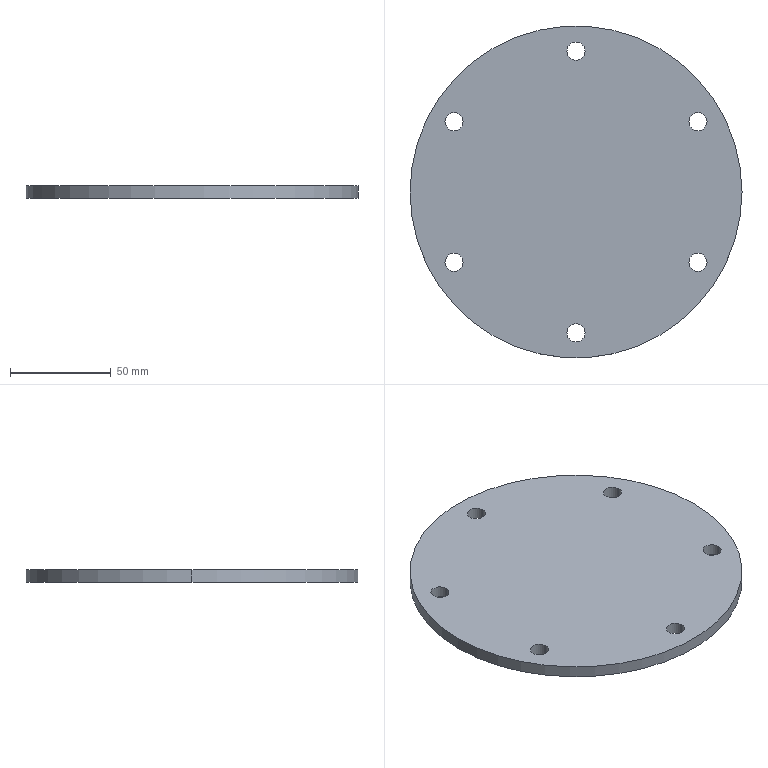Part | SolidWorks | features FlatPattern 1, SMBaseFlange 1, SheetMetal 1 | 1 solid | 16 faces | box 165 x 165 x 6 mm | volume 126005 mm3 | cylinder 14 | plane 2 | commonest cylinder face diameters 9 x12 165 x2
STEP:
#1=CARTESIAN_POINT('',(-65.122,35.,6.));
#2=VERTEX_POINT('',#1);
#3=CARTESIAN_POINT('',(-56.122,35.,6.));
#4=VERTEX_POINT('',#3);
#5=CARTESIAN_POINT('',(-60.622,35.,6.));
#6=DIRECTION('',(0.,0.,1.));
#7=DIRECTION('',(1.,0.,0.));
#8=AXIS2_PLACEMENT_3D('',#5,#6,#7);
#9=CIRCLE('',#8,4.5);
#10=EDGE_CURVE('',#2,#4,#9,.T.);
#11=ORIENTED_EDGE('',*,*,#10,.T.);
#12=CARTESIAN_POINT('',(-56.122,35.,0.));
#13=VERTEX_POINT('',#12);
#14=CARTESIAN_POINT('',(-56.122,35.,6.));
#15=DIRECTION('',(0.,0.,-1.));
#16=VECTOR('',#15,1000.);
#17=LINE('',#14,#16);
#18=EDGE_CURVE('',#4,#13,#17,.T.);
#19=ORIENTED_EDGE('',*,*,#18,.T.);
#20=CARTESIAN_POINT('',(-65.122,35.,0.));
#21=VERTEX_POINT('',#20);
#22=CARTESIAN_POINT('',(-60.622,35.,0.));
#23=DIRECTION('',(0.,0.,1.));
#24=DIRECTION('',(1.,0.,0.));
#25=AXIS2_PLACEMENT_3D('',#22,#23,#24);
#26=CIRCLE('',#25,4.5);
#27=EDGE_CURVE('',#21,#13,#26,.T.);
#28=ORIENTED_EDGE('',*,*,#27,.F.);
#29=CARTESIAN_POINT('',(-65.122,35.,6.));
#30=DIRECTION('',(0.,0.,-1.));
#31=VECTOR('',#30,1000.);
#32=LINE('',#29,#31);
#33=EDGE_CURVE('',#2,#21,#32,.T.);
#34=ORIENTED_EDGE('',*,*,#33,.F.);
#35=EDGE_LOOP('',(#11,#19,#28,#34));
#36=FACE_OUTER_BOUND('',#35,.T.);
#37=CARTESIAN_POINT('',(-60.622,35.,6.));
#38=DIRECTION('',(0.,0.,-1.));
#39=DIRECTION('',(-1.,0.,0.));
#40=AXIS2_PLACEMENT_3D('',#37,#38,#39);
#41=CYLINDRICAL_SURFACE('',#40,4.5);
#42=ADVANCED_FACE('',(#36),#41,.F.);
#43=CARTESIAN_POINT('',(-65.122,-35.,6.));
#44=VERTEX_POINT('',#43);
#45=CARTESIAN_POINT('',(-56.122,-35.,6.));
#46=VERTEX_POINT('',#45);
#47=CARTESIAN_POINT('',(-60.622,-35.,6.));
#48=DIRECTION('',(0.,0.,1.));
#49=DIRECTION('',(1.,0.,0.));
#50=AXIS2_PLACEMENT_3D('',#47,#48,#49);
#51=CIRCLE('',#50,4.5);
#52=EDGE_CURVE('',#44,#46,#51,.T.);
#53=ORIENTED_EDGE('',*,*,#52,.T.);
#54=CARTESIAN_POINT('',(-56.122,-35.,0.));
#55=VERTEX_POINT('',#54);
#56=CARTESIAN_POINT('',(-56.122,-35.,6.));
#57=DIRECTION('',(0.,0.,-1.));
#58=VECTOR('',#57,1000.);
#59=LINE('',#56,#58);
#60=EDGE_CURVE('',#46,#55,#59,.T.);
#61=ORIENTED_EDGE('',*,*,#60,.T.);
#62=CARTESIAN_POINT('',(-65.122,-35.,0.));
#63=VERTEX_POINT('',#62);
#64=CARTESIAN_POINT('',(-60.622,-35.,0.));
#65=DIRECTION('',(0.,0.,1.));
#66=DIRECTION('',(1.,0.,0.));
#67=AXIS2_PLACEMENT_3D('',#64,#65,#66);
#68=CIRCLE('',#67,4.5);
#69=EDGE_CURVE('',#63,#55,#68,.T.);
#70=ORIENTED_EDGE('',*,*,#69,.F.);
#71=CARTESIAN_POINT('',(-65.122,-35.,6.));
#72=DIRECTION('',(0.,0.,-1.));
#73=VECTOR('',#72,1000.);
#74=LINE('',#71,#73);
#75=EDGE_CURVE('',#44,#63,#74,.T.);
#76=ORIENTED_EDGE('',*,*,#75,.F.);
#77=EDGE_LOOP('',(#53,#61,#70,#76));
#78=FACE_OUTER_BOUND('',#77,.T.);
#79=CARTESIAN_POINT('',(-60.622,-35.,6.));
#80=DIRECTION('',(0.,0.,-1.));
#81=DIRECTION('',(-1.,0.,0.));
#82=AXIS2_PLACEMENT_3D('',#79,#80,#81);
#83=CYLINDRICAL_SURFACE('',#82,4.5);
#84=ADVANCED_FACE('',(#78),#83,.F.);
#85=CARTESIAN_POINT('',(-4.5,-70.,6.));
#86=VERTEX_POINT('',#85);
#87=CARTESIAN_POINT('',(4.5,-70.,6.));
#88=VERTEX_POINT('',#87);
#89=CARTESIAN_POINT('',(0.,-70.,6.));
#90=DIRECTION('',(0.,0.,1.));
#91=DIRECTION('',(1.,0.,0.));
#92=AXIS2_PLACEMENT_3D('',#89,#90,#91);
#93=CIRCLE('',#92,4.5);
#94=EDGE_CURVE('',#86,#88,#93,.T.);
#95=ORIENTED_EDGE('',*,*,#94,.T.);
#96=CARTESIAN_POINT('',(4.5,-70.,0.));
#97=VERTEX_POINT('',#96);
#98=CARTESIAN_POINT('',(4.5,-70.,6.));
#99=DIRECTION('',(0.,0.,-1.));
#100=VECTOR('',#99,1000.);
#101=LINE('',#98,#100);
#102=EDGE_CURVE('',#88,#97,#101,.T.);
#103=ORIENTED_EDGE('',*,*,#102,.T.);
#104=CARTESIAN_POINT('',(-4.5,-70.,0.));
#105=VERTEX_POINT('',#104);
#106=CARTESIAN_POINT('',(0.,-70.,0.));
#107=DIRECTION('',(0.,0.,1.));
#108=DIRECTION('',(1.,0.,0.));
#109=AXIS2_PLACEMENT_3D('',#106,#107,#108);
#110=CIRCLE('',#109,4.5);
#111=EDGE_CURVE('',#105,#97,#110,.T.);
#112=ORIENTED_EDGE('',*,*,#111,.F.);
#113=CARTESIAN_POINT('',(-4.5,-70.,6.));
#114=DIRECTION('',(0.,0.,-1.));
#115=VECTOR('',#114,1000.);
#116=LINE('',#113,#115);
#117=EDGE_CURVE('',#86,#105,#116,.T.);
#118=ORIENTED_EDGE('',*,*,#117,.F.);
#119=EDGE_LOOP('',(#95,#103,#112,#118));
#120=FACE_OUTER_BOUND('',#119,.T.);
#121=CARTESIAN_POINT('',(0.,-70.,6.));
#122=DIRECTION('',(0.,0.,-1.));
#123=DIRECTION('',(-1.,0.,0.));
#124=AXIS2_PLACEMENT_3D('',#121,#122,#123);
#125=CYLINDRICAL_SURFACE('',#124,4.5);
#126=ADVANCED_FACE('',(#120),#125,.F.);
#127=CARTESIAN_POINT('',(56.122,-35.,6.));
#128=VERTEX_POINT('',#127);
#129=CARTESIAN_POINT('',(65.122,-35.,6.));
#130=VERTEX_POINT('',#129);
#131=CARTESIAN_POINT('',(60.622,-35.,6.));
#132=DIRECTION('',(0.,0.,1.));
#133=DIRECTION('',(1.,0.,0.));
#134=AXIS2_PLACEMENT_3D('',#131,#132,#133);
#135=CIRCLE('',#134,4.5);
#136=EDGE_CURVE('',#128,#130,#135,.T.);
#137=ORIENTED_EDGE('',*,*,#136,.T.);
#138=CARTESIAN_POINT('',(65.122,-35.,0.));
#139=VERTEX_POINT('',#138);
#140=CARTESIAN_POINT('',(65.122,-35.,6.));
#141=DIRECTION('',(0.,0.,-1.));
#142=VECTOR('',#141,1000.);
#143=LINE('',#140,#142);
#144=EDGE_CURVE('',#130,#139,#143,.T.);
#145=ORIENTED_EDGE('',*,*,#144,.T.);
#146=CARTESIAN_POINT('',(56.122,-35.,0.));
#147=VERTEX_POINT('',#146);
#148=CARTESIAN_POINT('',(60.622,-35.,0.));
#149=DIRECTION('',(0.,0.,1.));
#150=DIRECTION('',(1.,0.,0.));
#151=AXIS2_PLACEMENT_3D('',#148,#149,#150);
#152=CIRCLE('',#151,4.5);
#153=EDGE_CURVE('',#147,#139,#152,.T.);
#154=ORIENTED_EDGE('',*,*,#153,.F.);
#155=CARTESIAN_POINT('',(56.122,-35.,6.));
#156=DIRECTION('',(0.,0.,-1.));
#157=VECTOR('',#156,1000.);
#158=LINE('',#155,#157);
#159=EDGE_CURVE('',#128,#147,#158,.T.);
#160=ORIENTED_EDGE('',*,*,#159,.F.);
#161=EDGE_LOOP('',(#137,#145,#154,#160));
#162=FACE_OUTER_BOUND('',#161,.T.);
#163=CARTESIAN_POINT('',(60.622,-35.,6.));
#164=DIRECTION('',(0.,0.,-1.));
#165=DIRECTION('',(-1.,0.,0.));
#166=AXIS2_PLACEMENT_3D('',#163,#164,#165);
#167=CYLINDRICAL_SURFACE('',#166,4.5);
#168=ADVANCED_FACE('',(#162),#167,.F.);
#169=CARTESIAN_POINT('',(56.122,35.,6.));
#170=VERTEX_POINT('',#169);
#171=CARTESIAN_POINT('',(65.122,35.,6.));
#172=VERTEX_POINT('',#171);
#173=CARTESIAN_POINT('',(60.622,35.,6.));
#174=DIRECTION('',(0.,0.,1.));
#175=DIRECTION('',(1.,0.,0.));
#176=AXIS2_PLACEMENT_3D('',#173,#174,#175);
#177=CIRCLE('',#176,4.5);
#178=EDGE_CURVE('',#170,#172,#177,.T.);
#179=ORIENTED_EDGE('',*,*,#178,.T.);
#180=CARTESIAN_POINT('',(65.122,35.,0.));
#181=VERTEX_POINT('',#180);
#182=CARTESIAN_POINT('',(65.122,35.,6.));
#183=DIRECTION('',(0.,0.,-1.));
#184=VECTOR('',#183,1000.);
#185=LINE('',#182,#184);
#186=EDGE_CURVE('',#172,#181,#185,.T.);
#187=ORIENTED_EDGE('',*,*,#186,.T.);
#188=CARTESIAN_POINT('',(56.122,35.,0.));
#189=VERTEX_POINT('',#188);
#190=CARTESIAN_POINT('',(60.622,35.,0.));
#191=DIRECTION('',(0.,0.,1.));
#192=DIRECTION('',(1.,0.,0.));
#193=AXIS2_PLACEMENT_3D('',#190,#191,#192);
#194=CIRCLE('',#193,4.5);
#195=EDGE_CURVE('',#189,#181,#194,.T.);
#196=ORIENTED_EDGE('',*,*,#195,.F.);
#197=CARTESIAN_POINT('',(56.122,35.,6.));
#198=DIRECTION('',(0.,0.,-1.));
#199=VECTOR('',#198,1000.);
#200=LINE('',#197,#199);
#201=EDGE_CURVE('',#170,#189,#200,.T.);
#202=ORIENTED_EDGE('',*,*,#201,.F.);
#203=EDGE_LOOP('',(#179,#187,#196,#202));
#204=FACE_OUTER_BOUND('',#203,.T.);
#205=CARTESIAN_POINT('',(60.622,35.,6.));
#206=DIRECTION('',(0.,0.,-1.));
#207=DIRECTION('',(-1.,0.,0.));
#208=AXIS2_PLACEMENT_3D('',#205,#206,#207);
#209=CYLINDRICAL_SURFACE('',#208,4.5);
#210=ADVANCED_FACE('',(#204),#209,.F.);
#211=CARTESIAN_POINT('',(-4.5,70.,6.));
#212=VERTEX_POINT('',#211);
#213=CARTESIAN_POINT('',(4.5,70.,6.));
#214=VERTEX_POINT('',#213);
#215=CARTESIAN_POINT('',(0.,70.,6.));
#216=DIRECTION('',(0.,0.,1.));
#217=DIRECTION('',(1.,0.,0.));
#218=AXIS2_PLACEMENT_3D('',#215,#216,#217);
#219=CIRCLE('',#218,4.5);
#220=EDGE_CURVE('',#212,#214,#219,.T.);
#221=ORIENTED_EDGE('',*,*,#220,.T.);
#222=CARTESIAN_POINT('',(4.5,70.,0.));
#223=VERTEX_POINT('',#222);
#224=CARTESIAN_POINT('',(4.5,70.,6.));
#225=DIRECTION('',(0.,0.,-1.));
#226=VECTOR('',#225,1000.);
#227=LINE('',#224,#226);
#228=EDGE_CURVE('',#214,#223,#227,.T.);
#229=ORIENTED_EDGE('',*,*,#228,.T.);
#230=CARTESIAN_POINT('',(-4.5,70.,0.));
#231=VERTEX_POINT('',#230);
#232=CARTESIAN_POINT('',(0.,70.,0.));
#233=DIRECTION('',(0.,0.,1.));
#234=DIRECTION('',(1.,0.,0.));
#235=AXIS2_PLACEMENT_3D('',#232,#233,#234);
#236=CIRCLE('',#235,4.5);
#237=EDGE_CURVE('',#231,#223,#236,.T.);
#238=ORIENTED_EDGE('',*,*,#237,.F.);
#239=CARTESIAN_POINT('',(-4.5,70.,6.));
#240=DIRECTION('',(0.,0.,-1.));
#241=VECTOR('',#240,1000.);
#242=LINE('',#239,#241);
#243=EDGE_CURVE('',#212,#231,#242,.T.);
#244=ORIENTED_EDGE('',*,*,#243,.F.);
#245=EDGE_LOOP('',(#221,#229,#238,#244));
#246=FACE_OUTER_BOUND('',#245,.T.);
#247=CARTESIAN_POINT('',(0.,70.,6.));
#248=DIRECTION('',(0.,0.,-1.));
#249=DIRECTION('',(-1.,0.,0.));
#250=AXIS2_PLACEMENT_3D('',#247,#248,#249);
#251=CYLINDRICAL_SURFACE('',#250,4.5);
#252=ADVANCED_FACE('',(#246),#251,.F.);
#253=CARTESIAN_POINT('',(82.5,0.,6.));
#254=VERTEX_POINT('',#253);
#255=CARTESIAN_POINT('',(-82.5,0.,6.));
#256=VERTEX_POINT('',#255);
#257=CARTESIAN_POINT('',(0.,0.,6.));
#258=DIRECTION('',(0.,0.,1.));
#259=DIRECTION('',(1.,0.,0.));
#260=AXIS2_PLACEMENT_3D('',#257,#258,#259);
#261=CIRCLE('',#260,82.5);
#262=EDGE_CURVE('',#254,#256,#261,.T.);
#263=ORIENTED_EDGE('',*,*,#262,.F.);
#264=CARTESIAN_POINT('',(82.5,0.,0.));
#265=VERTEX_POINT('',#264);
#266=CARTESIAN_POINT('',(82.5,0.,6.));
#267=DIRECTION('',(0.,0.,-1.));
#268=VECTOR('',#267,1000.);
#269=LINE('',#266,#268);
#270=EDGE_CURVE('',#254,#265,#269,.T.);
#271=ORIENTED_EDGE('',*,*,#270,.T.);
#272=CARTESIAN_POINT('',(-82.5,0.,0.));
#273=VERTEX_POINT('',#272);
#274=CARTESIAN_POINT('',(0.,0.,0.));
#275=DIRECTION('',(0.,0.,1.));
#276=DIRECTION('',(1.,0.,0.));
#277=AXIS2_PLACEMENT_3D('',#274,#275,#276);
#278=CIRCLE('',#277,82.5);
#279=EDGE_CURVE('',#265,#273,#278,.T.);
#280=ORIENTED_EDGE('',*,*,#279,.T.);
#281=CARTESIAN_POINT('',(-82.5,0.,6.));
#282=DIRECTION('',(0.,0.,-1.));
#283=VECTOR('',#282,1000.);
#284=LINE('',#281,#283);
#285=EDGE_CURVE('',#256,#273,#284,.T.);
#286=ORIENTED_EDGE('',*,*,#285,.F.);
#287=EDGE_LOOP('',(#263,#271,#280,#286));
#288=FACE_OUTER_BOUND('',#287,.T.);
#289=CARTESIAN_POINT('',(0.,0.,6.));
#290=DIRECTION('',(0.,0.,-1.));
#291=DIRECTION('',(-1.,0.,0.));
#292=AXIS2_PLACEMENT_3D('',#289,#290,#291);
#293=CYLINDRICAL_SURFACE('',#292,82.5);
#294=ADVANCED_FACE('',(#288),#293,.T.);
#295=ORIENTED_EDGE('',*,*,#52,.F.);
#296=CARTESIAN_POINT('',(-60.622,-35.,6.));
#297=DIRECTION('',(0.,0.,1.));
#298=DIRECTION('',(1.,0.,0.));
#299=AXIS2_PLACEMENT_3D('',#296,#297,#298);
#300=CIRCLE('',#299,4.5);
#301=EDGE_CURVE('',#46,#44,#300,.T.);
#302=ORIENTED_EDGE('',*,*,#301,.F.);
#303=EDGE_LOOP('',(#295,#302));
#304=FACE_BOUND('',#303,.T.);
#305=ORIENTED_EDGE('',*,*,#136,.F.);
#306=CARTESIAN_POINT('',(60.622,-35.,6.));
#307=DIRECTION('',(0.,0.,1.));
#308=DIRECTION('',(1.,0.,0.));
#309=AXIS2_PLACEMENT_3D('',#306,#307,#308);
#310=CIRCLE('',#309,4.5);
#311=EDGE_CURVE('',#130,#128,#310,.T.);
#312=ORIENTED_EDGE('',*,*,#311,.F.);
#313=EDGE_LOOP('',(#305,#312));
#314=FACE_BOUND('',#313,.T.);
#315=ORIENTED_EDGE('',*,*,#220,.F.);
#316=CARTESIAN_POINT('',(0.,70.,6.));
#317=DIRECTION('',(0.,0.,1.));
#318=DIRECTION('',(1.,0.,0.));
#319=AXIS2_PLACEMENT_3D('',#316,#317,#318);
#320=CIRCLE('',#319,4.5);
#321=EDGE_CURVE('',#214,#212,#320,.T.);
#322=ORIENTED_EDGE('',*,*,#321,.F.);
#323=EDGE_LOOP('',(#315,#322));
#324=FACE_BOUND('',#323,.T.);
#325=CARTESIAN_POINT('',(0.,0.,6.));
#326=DIRECTION('',(0.,0.,1.));
#327=DIRECTION('',(1.,0.,0.));
#328=AXIS2_PLACEMENT_3D('',#325,#326,#327);
#329=CIRCLE('',#328,82.5);
#330=EDGE_CURVE('',#256,#254,#329,.T.);
#331=ORIENTED_EDGE('',*,*,#330,.T.);
#332=ORIENTED_EDGE('',*,*,#262,.T.);
#333=EDGE_LOOP('',(#331,#332));
#334=FACE_OUTER_BOUND('',#333,.T.);
#335=ORIENTED_EDGE('',*,*,#178,.F.);
#336=CARTESIAN_POINT('',(60.622,35.,6.));
#337=DIRECTION('',(0.,0.,1.));
#338=DIRECTION('',(1.,0.,0.));
#339=AXIS2_PLACEMENT_3D('',#336,#337,#338);
#340=CIRCLE('',#339,4.5);
#341=EDGE_CURVE('',#172,#170,#340,.T.);
#342=ORIENTED_EDGE('',*,*,#341,.F.);
#343=EDGE_LOOP('',(#335,#342));
#344=FACE_BOUND('',#343,.T.);
#345=ORIENTED_EDGE('',*,*,#94,.F.);
#346=CARTESIAN_POINT('',(0.,-70.,6.));
#347=DIRECTION('',(0.,0.,1.));
#348=DIRECTION('',(1.,0.,0.));
#349=AXIS2_PLACEMENT_3D('',#346,#347,#348);
#350=CIRCLE('',#349,4.5);
#351=EDGE_CURVE('',#88,#86,#350,.T.);
#352=ORIENTED_EDGE('',*,*,#351,.F.);
#353=EDGE_LOOP('',(#345,#352));
#354=FACE_BOUND('',#353,.T.);
#355=ORIENTED_EDGE('',*,*,#10,.F.);
#356=CARTESIAN_POINT('',(-60.622,35.,6.));
#357=DIRECTION('',(0.,0.,1.));
#358=DIRECTION('',(1.,0.,0.));
#359=AXIS2_PLACEMENT_3D('',#356,#357,#358);
#360=CIRCLE('',#359,4.5);
#361=EDGE_CURVE('',#4,#2,#360,.T.);
#362=ORIENTED_EDGE('',*,*,#361,.F.);
#363=EDGE_LOOP('',(#355,#362));
#364=FACE_BOUND('',#363,.T.);
#365=CARTESIAN_POINT('',(0.,0.,6.));
#366=DIRECTION('',(0.,0.,1.));
#367=DIRECTION('',(1.,0.,0.));
#368=AXIS2_PLACEMENT_3D('',#365,#366,#367);
#369=PLANE('',#368);
#370=ADVANCED_FACE('',(#304,#314,#324,#334,#344,#354,#364),#369,.T.);
#371=CARTESIAN_POINT('',(0.,0.,0.));
#372=DIRECTION('',(0.,0.,1.));
#373=DIRECTION('',(1.,0.,0.));
#374=AXIS2_PLACEMENT_3D('',#371,#372,#373);
#375=CIRCLE('',#374,82.5);
#376=EDGE_CURVE('',#273,#265,#375,.T.);
#377=ORIENTED_EDGE('',*,*,#376,.F.);
#378=ORIENTED_EDGE('',*,*,#279,.F.);
#379=EDGE_LOOP('',(#377,#378));
#380=FACE_OUTER_BOUND('',#379,.T.);
#381=ORIENTED_EDGE('',*,*,#237,.T.);
#382=CARTESIAN_POINT('',(0.,70.,0.));
#383=DIRECTION('',(0.,0.,1.));
#384=DIRECTION('',(1.,0.,0.));
#385=AXIS2_PLACEMENT_3D('',#382,#383,#384);
#386=CIRCLE('',#385,4.5);
#387=EDGE_CURVE('',#223,#231,#386,.T.);
#388=ORIENTED_EDGE('',*,*,#387,.T.);
#389=EDGE_LOOP('',(#381,#388));
#390=FACE_BOUND('',#389,.T.);
#391=ORIENTED_EDGE('',*,*,#195,.T.);
#392=CARTESIAN_POINT('',(60.622,35.,0.));
#393=DIRECTION('',(0.,0.,1.));
#394=DIRECTION('',(1.,0.,0.));
#395=AXIS2_PLACEMENT_3D('',#392,#393,#394);
#396=CIRCLE('',#395,4.5);
#397=EDGE_CURVE('',#181,#189,#396,.T.);
#398=ORIENTED_EDGE('',*,*,#397,.T.);
#399=EDGE_LOOP('',(#391,#398));
#400=FACE_BOUND('',#399,.T.);
#401=ORIENTED_EDGE('',*,*,#153,.T.);
#402=CARTESIAN_POINT('',(60.622,-35.,0.));
#403=DIRECTION('',(0.,0.,1.));
#404=DIRECTION('',(1.,0.,0.));
#405=AXIS2_PLACEMENT_3D('',#402,#403,#404);
#406=CIRCLE('',#405,4.5);
#407=EDGE_CURVE('',#139,#147,#406,.T.);
#408=ORIENTED_EDGE('',*,*,#407,.T.);
#409=EDGE_LOOP('',(#401,#408));
#410=FACE_BOUND('',#409,.T.);
#411=ORIENTED_EDGE('',*,*,#111,.T.);
#412=CARTESIAN_POINT('',(0.,-70.,0.));
#413=DIRECTION('',(0.,0.,1.));
#414=DIRECTION('',(1.,0.,0.));
#415=AXIS2_PLACEMENT_3D('',#412,#413,#414);
#416=CIRCLE('',#415,4.5);
#417=EDGE_CURVE('',#97,#105,#416,.T.);
#418=ORIENTED_EDGE('',*,*,#417,.T.);
#419=EDGE_LOOP('',(#411,#418));
#420=FACE_BOUND('',#419,.T.);
#421=ORIENTED_EDGE('',*,*,#69,.T.);
#422=CARTESIAN_POINT('',(-60.622,-35.,0.));
#423=DIRECTION('',(0.,0.,1.));
#424=DIRECTION('',(1.,0.,0.));
#425=AXIS2_PLACEMENT_3D('',#422,#423,#424);
#426=CIRCLE('',#425,4.5);
#427=EDGE_CURVE('',#55,#63,#426,.T.);
#428=ORIENTED_EDGE('',*,*,#427,.T.);
#429=EDGE_LOOP('',(#421,#428));
#430=FACE_BOUND('',#429,.T.);
#431=ORIENTED_EDGE('',*,*,#27,.T.);
#432=CARTESIAN_POINT('',(-60.622,35.,0.));
#433=DIRECTION('',(0.,0.,1.));
#434=DIRECTION('',(1.,0.,0.));
#435=AXIS2_PLACEMENT_3D('',#432,#433,#434);
#436=CIRCLE('',#435,4.5);
#437=EDGE_CURVE('',#13,#21,#436,.T.);
#438=ORIENTED_EDGE('',*,*,#437,.T.);
#439=EDGE_LOOP('',(#431,#438));
#440=FACE_BOUND('',#439,.T.);
#441=CARTESIAN_POINT('',(0.,0.,0.));
#442=DIRECTION('',(0.,0.,1.));
#443=DIRECTION('',(1.,0.,0.));
#444=AXIS2_PLACEMENT_3D('',#441,#442,#443);
#445=PLANE('',#444);
#446=ADVANCED_FACE('',(#380,#390,#400,#410,#420,#430,#440),#445,.F.);
#447=ORIENTED_EDGE('',*,*,#270,.F.);
#448=ORIENTED_EDGE('',*,*,#330,.F.);
#449=ORIENTED_EDGE('',*,*,#285,.T.);
#450=ORIENTED_EDGE('',*,*,#376,.T.);
#451=EDGE_LOOP('',(#447,#448,#449,#450));
#452=FACE_OUTER_BOUND('',#451,.T.);
#453=CARTESIAN_POINT('',(0.,0.,6.));
#454=DIRECTION('',(0.,0.,-1.));
#455=DIRECTION('',(-1.,0.,0.));
#456=AXIS2_PLACEMENT_3D('',#453,#454,#455);
#457=CYLINDRICAL_SURFACE('',#456,82.5);
#458=ADVANCED_FACE('',(#452),#457,.T.);
#459=ORIENTED_EDGE('',*,*,#228,.F.);
#460=ORIENTED_EDGE('',*,*,#321,.T.);
#461=ORIENTED_EDGE('',*,*,#243,.T.);
#462=ORIENTED_EDGE('',*,*,#387,.F.);
#463=EDGE_LOOP('',(#459,#460,#461,#462));
#464=FACE_OUTER_BOUND('',#463,.T.);
#465=CARTESIAN_POINT('',(0.,70.,6.));
#466=DIRECTION('',(0.,0.,-1.));
#467=DIRECTION('',(-1.,0.,0.));
#468=AXIS2_PLACEMENT_3D('',#465,#466,#467);
#469=CYLINDRICAL_SURFACE('',#468,4.5);
#470=ADVANCED_FACE('',(#464),#469,.F.);
#471=ORIENTED_EDGE('',*,*,#186,.F.);
#472=ORIENTED_EDGE('',*,*,#341,.T.);
#473=ORIENTED_EDGE('',*,*,#201,.T.);
#474=ORIENTED_EDGE('',*,*,#397,.F.);
#475=EDGE_LOOP('',(#471,#472,#473,#474));
#476=FACE_OUTER_BOUND('',#475,.T.);
#477=CARTESIAN_POINT('',(60.622,35.,6.));
#478=DIRECTION('',(0.,0.,-1.));
#479=DIRECTION('',(-1.,0.,0.));
#480=AXIS2_PLACEMENT_3D('',#477,#478,#479);
#481=CYLINDRICAL_SURFACE('',#480,4.5);
#482=ADVANCED_FACE('',(#476),#481,.F.);
#483=ORIENTED_EDGE('',*,*,#144,.F.);
#484=ORIENTED_EDGE('',*,*,#311,.T.);
#485=ORIENTED_EDGE('',*,*,#159,.T.);
#486=ORIENTED_EDGE('',*,*,#407,.F.);
#487=EDGE_LOOP('',(#483,#484,#485,#486));
#488=FACE_OUTER_BOUND('',#487,.T.);
#489=CARTESIAN_POINT('',(60.622,-35.,6.));
#490=DIRECTION('',(0.,0.,-1.));
#491=DIRECTION('',(-1.,0.,0.));
#492=AXIS2_PLACEMENT_3D('',#489,#490,#491);
#493=CYLINDRICAL_SURFACE('',#492,4.5);
#494=ADVANCED_FACE('',(#488),#493,.F.);
#495=ORIENTED_EDGE('',*,*,#102,.F.);
#496=ORIENTED_EDGE('',*,*,#351,.T.);
#497=ORIENTED_EDGE('',*,*,#117,.T.);
#498=ORIENTED_EDGE('',*,*,#417,.F.);
#499=EDGE_LOOP('',(#495,#496,#497,#498));
#500=FACE_OUTER_BOUND('',#499,.T.);
#501=CARTESIAN_POINT('',(0.,-70.,6.));
#502=DIRECTION('',(0.,0.,-1.));
#503=DIRECTION('',(-1.,0.,0.));
#504=AXIS2_PLACEMENT_3D('',#501,#502,#503);
#505=CYLINDRICAL_SURFACE('',#504,4.5);
#506=ADVANCED_FACE('',(#500),#505,.F.);
#507=ORIENTED_EDGE('',*,*,#60,.F.);
#508=ORIENTED_EDGE('',*,*,#301,.T.);
#509=ORIENTED_EDGE('',*,*,#75,.T.);
#510=ORIENTED_EDGE('',*,*,#427,.F.);
#511=EDGE_LOOP('',(#507,#508,#509,#510));
#512=FACE_OUTER_BOUND('',#511,.T.);
#513=CARTESIAN_POINT('',(-60.622,-35.,6.));
#514=DIRECTION('',(0.,0.,-1.));
#515=DIRECTION('',(-1.,0.,0.));
#516=AXIS2_PLACEMENT_3D('',#513,#514,#515);
#517=CYLINDRICAL_SURFACE('',#516,4.5);
#518=ADVANCED_FACE('',(#512),#517,.F.);
#519=ORIENTED_EDGE('',*,*,#18,.F.);
#520=ORIENTED_EDGE('',*,*,#361,.T.);
#521=ORIENTED_EDGE('',*,*,#33,.T.);
#522=ORIENTED_EDGE('',*,*,#437,.F.);
#523=EDGE_LOOP('',(#519,#520,#521,#522));
#524=FACE_OUTER_BOUND('',#523,.T.);
#525=CARTESIAN_POINT('',(-60.622,35.,6.));
#526=DIRECTION('',(0.,0.,-1.));
#527=DIRECTION('',(-1.,0.,0.));
#528=AXIS2_PLACEMENT_3D('',#525,#526,#527);
#529=CYLINDRICAL_SURFACE('',#528,4.5);
#530=ADVANCED_FACE('',(#524),#529,.F.);
#531=CLOSED_SHELL('',(#42,#84,#126,#168,#210,#252,#294,#370,#446,#458,#470,#482,#494,#506,#518,#530));
#532=MANIFOLD_SOLID_BREP('',#531);
#533=CARTESIAN_POINT('',(0.,0.,0.));
#534=DIRECTION('',(0.,0.,1.));
#535=DIRECTION('',(1.,0.,0.));
#536=AXIS2_PLACEMENT_3D('',#533,#534,#535);
#537=(LENGTH_UNIT()NAMED_UNIT(*)SI_UNIT(.MILLI.,.METRE.));
#538=UNCERTAINTY_MEASURE_WITH_UNIT(LENGTH_MEASURE(0.00001),#537,'','');
#539=(NAMED_UNIT(*)PLANE_ANGLE_UNIT()SI_UNIT($,.RADIAN.));
#540=(NAMED_UNIT(*)SI_UNIT($,.STERADIAN.)SOLID_ANGLE_UNIT());
#541=(GEOMETRIC_REPRESENTATION_CONTEXT(3)GLOBAL_UNCERTAINTY_ASSIGNED_CONTEXT((#538))GLOBAL_UNIT_ASSIGNED_CONTEXT((#537,#539,#540))REPRESENTATION_CONTEXT('',''));
#542=ADVANCED_BREP_SHAPE_REPRESENTATION('',(#532,#536),#541);